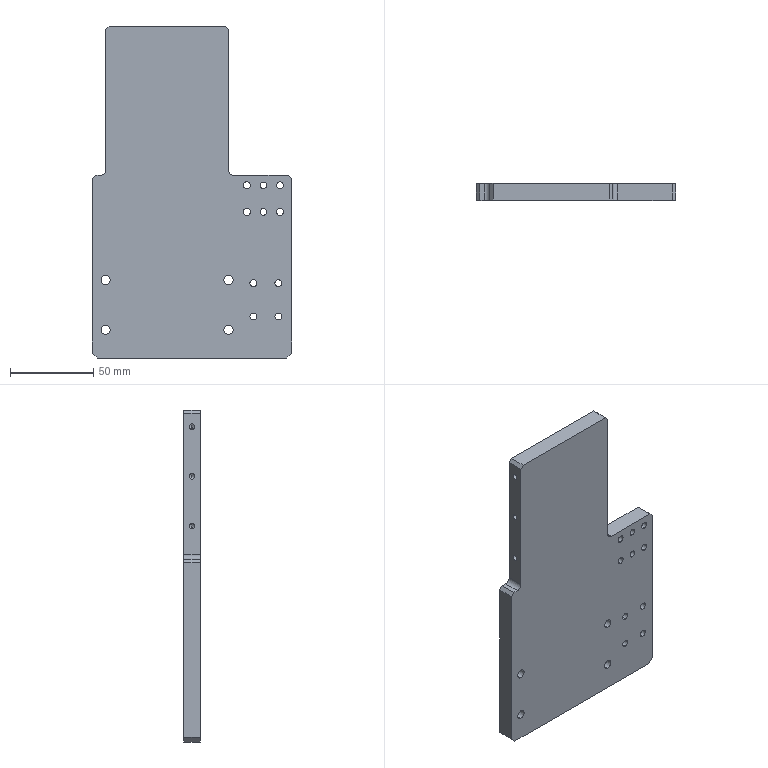Part | SolidWorks | features HoleWzd 6, Chamfer 2, Extrusion 1, Fillet 1, ICE 1 | 1 solid | 82 faces | box 120 x 10 x 200 mm | volume 194374 mm3 | cylinder 50 | plane 20 | cone 12 | commonest cylinder face diameters 4.2 x16 3.3 x12 5.5 x8 10 x8 4 x4 6 x2